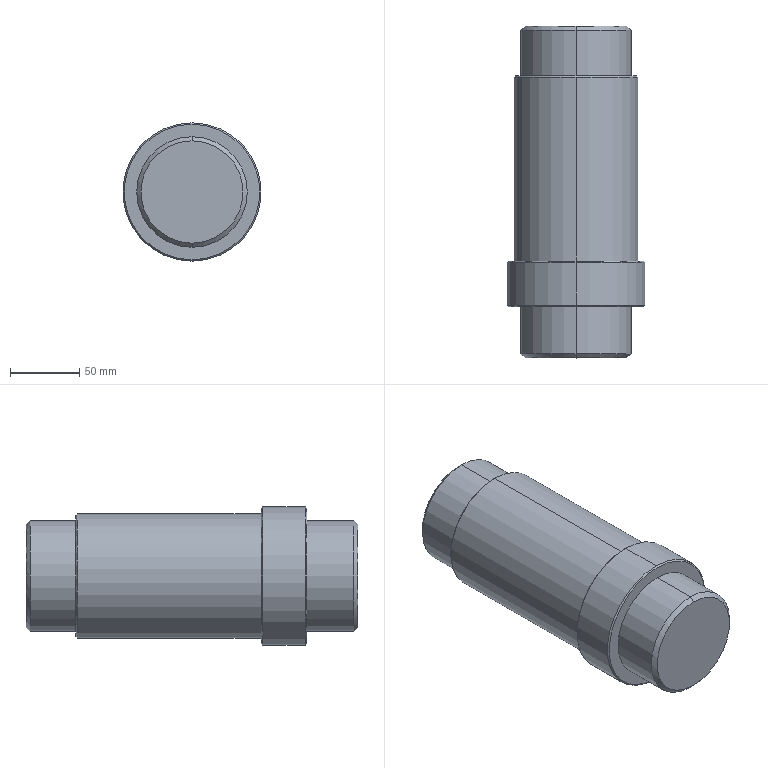Part | SolidWorks | features ICE 3, Chamfer 2, Extrusion 1 | 1 solid | 23 faces | box 100 x 240 x 100 mm | volume 1475933 mm3 | cone 10 | cylinder 8 | plane 5 | commonest cylinder face diameters 80 x4 90 x2 100 x2
STEP:
#1=CARTESIAN_POINT('',(0.,-50.,49.));
#2=VERTEX_POINT('',#1);
#3=CARTESIAN_POINT('',(0.,-50.,-49.));
#4=VERTEX_POINT('',#3);
#5=CARTESIAN_POINT('',(0.,-50.,0.));
#6=DIRECTION('',(0.,1.,0.));
#7=DIRECTION('',(0.,0.,1.));
#8=AXIS2_PLACEMENT_3D('',#5,#6,#7);
#9=CIRCLE('',#8,49.);
#10=EDGE_CURVE('',#2,#4,#9,.T.);
#11=ORIENTED_EDGE('',*,*,#10,.F.);
#12=CARTESIAN_POINT('',(0.,-51.,50.));
#13=VERTEX_POINT('',#12);
#14=CARTESIAN_POINT('',(0.,-50.,49.));
#15=DIRECTION('',(0.,-0.7071,0.7071));
#16=VECTOR('',#15,1000.);
#17=LINE('',#14,#16);
#18=EDGE_CURVE('',#2,#13,#17,.T.);
#19=ORIENTED_EDGE('',*,*,#18,.T.);
#20=CARTESIAN_POINT('',(0.,-51.,-50.));
#21=VERTEX_POINT('',#20);
#22=CARTESIAN_POINT('',(0.,-51.,0.));
#23=DIRECTION('',(0.,-1.,0.));
#24=DIRECTION('',(0.,0.,1.));
#25=AXIS2_PLACEMENT_3D('',#22,#23,#24);
#26=CIRCLE('',#25,50.);
#27=EDGE_CURVE('',#21,#13,#26,.T.);
#28=ORIENTED_EDGE('',*,*,#27,.F.);
#29=CARTESIAN_POINT('',(0.,-50.,-49.));
#30=DIRECTION('',(0.,-0.7071,-0.7071));
#31=VECTOR('',#30,1000.);
#32=LINE('',#29,#31);
#33=EDGE_CURVE('',#4,#21,#32,.T.);
#34=ORIENTED_EDGE('',*,*,#33,.F.);
#35=EDGE_LOOP('',(#11,#19,#28,#34));
#36=FACE_OUTER_BOUND('',#35,.T.);
#37=CARTESIAN_POINT('',(0.,-50.,0.));
#38=DIRECTION('',(0.,-1.,0.));
#39=DIRECTION('',(0.,0.,-1.));
#40=AXIS2_PLACEMENT_3D('',#37,#38,#39);
#41=CONICAL_SURFACE('',#40,49.,0.7854);
#42=ADVANCED_FACE('',(#36),#41,.T.);
#43=CARTESIAN_POINT('',(0.,-83.,-49.));
#44=VERTEX_POINT('',#43);
#45=CARTESIAN_POINT('',(0.,-83.,49.));
#46=VERTEX_POINT('',#45);
#47=CARTESIAN_POINT('',(0.,-83.,0.));
#48=DIRECTION('',(0.,-1.,0.));
#49=DIRECTION('',(0.,0.,-1.));
#50=AXIS2_PLACEMENT_3D('',#47,#48,#49);
#51=CIRCLE('',#50,49.);
#52=EDGE_CURVE('',#44,#46,#51,.T.);
#53=ORIENTED_EDGE('',*,*,#52,.F.);
#54=CARTESIAN_POINT('',(0.,-82.,-50.));
#55=VERTEX_POINT('',#54);
#56=CARTESIAN_POINT('',(0.,-83.,-49.));
#57=DIRECTION('',(0.,0.7071,-0.7071));
#58=VECTOR('',#57,1000.);
#59=LINE('',#56,#58);
#60=EDGE_CURVE('',#44,#55,#59,.T.);
#61=ORIENTED_EDGE('',*,*,#60,.T.);
#62=CARTESIAN_POINT('',(0.,-82.,50.));
#63=VERTEX_POINT('',#62);
#64=CARTESIAN_POINT('',(0.,-82.,0.));
#65=DIRECTION('',(0.,1.,0.));
#66=DIRECTION('',(0.,0.,-1.));
#67=AXIS2_PLACEMENT_3D('',#64,#65,#66);
#68=CIRCLE('',#67,50.);
#69=EDGE_CURVE('',#63,#55,#68,.T.);
#70=ORIENTED_EDGE('',*,*,#69,.F.);
#71=CARTESIAN_POINT('',(0.,-83.,49.));
#72=DIRECTION('',(0.,0.7071,0.7071));
#73=VECTOR('',#72,1000.);
#74=LINE('',#71,#73);
#75=EDGE_CURVE('',#46,#63,#74,.T.);
#76=ORIENTED_EDGE('',*,*,#75,.F.);
#77=EDGE_LOOP('',(#53,#61,#70,#76));
#78=FACE_OUTER_BOUND('',#77,.T.);
#79=CARTESIAN_POINT('',(0.,-83.,0.));
#80=DIRECTION('',(0.,1.,0.));
#81=DIRECTION('',(0.,0.,1.));
#82=AXIS2_PLACEMENT_3D('',#79,#80,#81);
#83=CONICAL_SURFACE('',#82,49.,0.7854);
#84=ADVANCED_FACE('',(#78),#83,.T.);
#85=CARTESIAN_POINT('',(0.,84.,44.));
#86=VERTEX_POINT('',#85);
#87=CARTESIAN_POINT('',(0.,84.,-44.));
#88=VERTEX_POINT('',#87);
#89=CARTESIAN_POINT('',(0.,84.,0.));
#90=DIRECTION('',(0.,1.,0.));
#91=DIRECTION('',(0.,0.,1.));
#92=AXIS2_PLACEMENT_3D('',#89,#90,#91);
#93=CIRCLE('',#92,44.);
#94=EDGE_CURVE('',#86,#88,#93,.T.);
#95=ORIENTED_EDGE('',*,*,#94,.F.);
#96=CARTESIAN_POINT('',(0.,83.,45.));
#97=VERTEX_POINT('',#96);
#98=CARTESIAN_POINT('',(0.,84.,44.));
#99=DIRECTION('',(0.,-0.7071,0.7071));
#100=VECTOR('',#99,1000.);
#101=LINE('',#98,#100);
#102=EDGE_CURVE('',#86,#97,#101,.T.);
#103=ORIENTED_EDGE('',*,*,#102,.T.);
#104=CARTESIAN_POINT('',(0.,83.,-45.));
#105=VERTEX_POINT('',#104);
#106=CARTESIAN_POINT('',(0.,83.,0.));
#107=DIRECTION('',(0.,-1.,0.));
#108=DIRECTION('',(0.,0.,1.));
#109=AXIS2_PLACEMENT_3D('',#106,#107,#108);
#110=CIRCLE('',#109,45.);
#111=EDGE_CURVE('',#105,#97,#110,.T.);
#112=ORIENTED_EDGE('',*,*,#111,.F.);
#113=CARTESIAN_POINT('',(0.,84.,-44.));
#114=DIRECTION('',(0.,-0.7071,-0.7071));
#115=VECTOR('',#114,1000.);
#116=LINE('',#113,#115);
#117=EDGE_CURVE('',#88,#105,#116,.T.);
#118=ORIENTED_EDGE('',*,*,#117,.F.);
#119=EDGE_LOOP('',(#95,#103,#112,#118));
#120=FACE_OUTER_BOUND('',#119,.T.);
#121=CARTESIAN_POINT('',(0.,84.,0.));
#122=DIRECTION('',(0.,-1.,0.));
#123=DIRECTION('',(0.,0.,-1.));
#124=AXIS2_PLACEMENT_3D('',#121,#122,#123);
#125=CONICAL_SURFACE('',#124,44.,0.7854);
#126=ADVANCED_FACE('',(#120),#125,.T.);
#127=CARTESIAN_POINT('',(0.,120.,37.));
#128=VERTEX_POINT('',#127);
#129=CARTESIAN_POINT('',(0.,120.,-37.));
#130=VERTEX_POINT('',#129);
#131=CARTESIAN_POINT('',(0.,120.,0.));
#132=DIRECTION('',(0.,1.,0.));
#133=DIRECTION('',(0.,0.,1.));
#134=AXIS2_PLACEMENT_3D('',#131,#132,#133);
#135=CIRCLE('',#134,37.);
#136=EDGE_CURVE('',#128,#130,#135,.T.);
#137=ORIENTED_EDGE('',*,*,#136,.F.);
#138=CARTESIAN_POINT('',(0.,117.,40.));
#139=VERTEX_POINT('',#138);
#140=CARTESIAN_POINT('',(0.,120.,37.));
#141=DIRECTION('',(0.,-0.7071,0.7071));
#142=VECTOR('',#141,1000.);
#143=LINE('',#140,#142);
#144=EDGE_CURVE('',#128,#139,#143,.T.);
#145=ORIENTED_EDGE('',*,*,#144,.T.);
#146=CARTESIAN_POINT('',(0.,117.,-40.));
#147=VERTEX_POINT('',#146);
#148=CARTESIAN_POINT('',(0.,117.,0.));
#149=DIRECTION('',(0.,-1.,0.));
#150=DIRECTION('',(0.,0.,1.));
#151=AXIS2_PLACEMENT_3D('',#148,#149,#150);
#152=CIRCLE('',#151,40.);
#153=EDGE_CURVE('',#147,#139,#152,.T.);
#154=ORIENTED_EDGE('',*,*,#153,.F.);
#155=CARTESIAN_POINT('',(0.,120.,-37.));
#156=DIRECTION('',(0.,-0.7071,-0.7071));
#157=VECTOR('',#156,1000.);
#158=LINE('',#155,#157);
#159=EDGE_CURVE('',#130,#147,#158,.T.);
#160=ORIENTED_EDGE('',*,*,#159,.F.);
#161=EDGE_LOOP('',(#137,#145,#154,#160));
#162=FACE_OUTER_BOUND('',#161,.T.);
#163=CARTESIAN_POINT('',(0.,120.,0.));
#164=DIRECTION('',(0.,-1.,0.));
#165=DIRECTION('',(0.,0.,-1.));
#166=AXIS2_PLACEMENT_3D('',#163,#164,#165);
#167=CONICAL_SURFACE('',#166,37.,0.7854);
#168=ADVANCED_FACE('',(#162),#167,.T.);
#169=CARTESIAN_POINT('',(0.,-120.,-37.));
#170=VERTEX_POINT('',#169);
#171=CARTESIAN_POINT('',(0.,-120.,37.));
#172=VERTEX_POINT('',#171);
#173=CARTESIAN_POINT('',(0.,-120.,0.));
#174=DIRECTION('',(0.,-1.,0.));
#175=DIRECTION('',(0.,0.,1.));
#176=AXIS2_PLACEMENT_3D('',#173,#174,#175);
#177=CIRCLE('',#176,37.);
#178=EDGE_CURVE('',#170,#172,#177,.T.);
#179=ORIENTED_EDGE('',*,*,#178,.F.);
#180=CARTESIAN_POINT('',(0.,-117.,-40.));
#181=VERTEX_POINT('',#180);
#182=CARTESIAN_POINT('',(0.,-120.,-37.));
#183=DIRECTION('',(0.,0.7071,-0.7071));
#184=VECTOR('',#183,1000.);
#185=LINE('',#182,#184);
#186=EDGE_CURVE('',#170,#181,#185,.T.);
#187=ORIENTED_EDGE('',*,*,#186,.T.);
#188=CARTESIAN_POINT('',(0.,-117.,40.));
#189=VERTEX_POINT('',#188);
#190=CARTESIAN_POINT('',(0.,-117.,0.));
#191=DIRECTION('',(0.,1.,0.));
#192=DIRECTION('',(0.,0.,1.));
#193=AXIS2_PLACEMENT_3D('',#190,#191,#192);
#194=CIRCLE('',#193,40.);
#195=EDGE_CURVE('',#189,#181,#194,.T.);
#196=ORIENTED_EDGE('',*,*,#195,.F.);
#197=CARTESIAN_POINT('',(0.,-120.,37.));
#198=DIRECTION('',(0.,0.7071,0.7071));
#199=VECTOR('',#198,1000.);
#200=LINE('',#197,#199);
#201=EDGE_CURVE('',#172,#189,#200,.T.);
#202=ORIENTED_EDGE('',*,*,#201,.F.);
#203=EDGE_LOOP('',(#179,#187,#196,#202));
#204=FACE_OUTER_BOUND('',#203,.T.);
#205=CARTESIAN_POINT('',(0.,-120.,0.));
#206=DIRECTION('',(0.,1.,0.));
#207=DIRECTION('',(0.,0.,1.));
#208=AXIS2_PLACEMENT_3D('',#205,#206,#207);
#209=CONICAL_SURFACE('',#208,37.,0.7854);
#210=ADVANCED_FACE('',(#204),#209,.T.);
#211=CARTESIAN_POINT('',(0.,84.,40.));
#212=VERTEX_POINT('',#211);
#213=CARTESIAN_POINT('',(0.,84.,-40.));
#214=VERTEX_POINT('',#213);
#215=CARTESIAN_POINT('',(0.,84.,0.));
#216=DIRECTION('',(0.,1.,0.));
#217=DIRECTION('',(0.,0.,1.));
#218=AXIS2_PLACEMENT_3D('',#215,#216,#217);
#219=CIRCLE('',#218,40.);
#220=EDGE_CURVE('',#212,#214,#219,.T.);
#221=ORIENTED_EDGE('',*,*,#220,.T.);
#222=CARTESIAN_POINT('',(0.,84.,-40.));
#223=DIRECTION('',(0.,1.,0.));
#224=VECTOR('',#223,1000.);
#225=LINE('',#222,#224);
#226=EDGE_CURVE('',#214,#147,#225,.T.);
#227=ORIENTED_EDGE('',*,*,#226,.T.);
#228=ORIENTED_EDGE('',*,*,#153,.T.);
#229=CARTESIAN_POINT('',(0.,84.,40.));
#230=DIRECTION('',(0.,1.,0.));
#231=VECTOR('',#230,1000.);
#232=LINE('',#229,#231);
#233=EDGE_CURVE('',#212,#139,#232,.T.);
#234=ORIENTED_EDGE('',*,*,#233,.F.);
#235=EDGE_LOOP('',(#221,#227,#228,#234));
#236=FACE_OUTER_BOUND('',#235,.T.);
#237=CARTESIAN_POINT('',(0.,84.,0.));
#238=DIRECTION('',(0.,1.,0.));
#239=DIRECTION('',(0.,0.,1.));
#240=AXIS2_PLACEMENT_3D('',#237,#238,#239);
#241=CYLINDRICAL_SURFACE('',#240,40.);
#242=ADVANCED_FACE('',(#236),#241,.T.);
#243=CARTESIAN_POINT('',(0.,-50.,45.));
#244=VERTEX_POINT('',#243);
#245=CARTESIAN_POINT('',(0.,-50.,-45.));
#246=VERTEX_POINT('',#245);
#247=CARTESIAN_POINT('',(0.,-50.,0.));
#248=DIRECTION('',(0.,1.,0.));
#249=DIRECTION('',(0.,0.,1.));
#250=AXIS2_PLACEMENT_3D('',#247,#248,#249);
#251=CIRCLE('',#250,45.);
#252=EDGE_CURVE('',#244,#246,#251,.T.);
#253=ORIENTED_EDGE('',*,*,#252,.T.);
#254=CARTESIAN_POINT('',(0.,-50.,-45.));
#255=DIRECTION('',(0.,1.,0.));
#256=VECTOR('',#255,1000.);
#257=LINE('',#254,#256);
#258=EDGE_CURVE('',#246,#105,#257,.T.);
#259=ORIENTED_EDGE('',*,*,#258,.T.);
#260=ORIENTED_EDGE('',*,*,#111,.T.);
#261=CARTESIAN_POINT('',(0.,-50.,45.));
#262=DIRECTION('',(0.,1.,0.));
#263=VECTOR('',#262,1000.);
#264=LINE('',#261,#263);
#265=EDGE_CURVE('',#244,#97,#264,.T.);
#266=ORIENTED_EDGE('',*,*,#265,.F.);
#267=EDGE_LOOP('',(#253,#259,#260,#266));
#268=FACE_OUTER_BOUND('',#267,.T.);
#269=CARTESIAN_POINT('',(0.,-50.,0.));
#270=DIRECTION('',(0.,1.,0.));
#271=DIRECTION('',(0.,0.,1.));
#272=AXIS2_PLACEMENT_3D('',#269,#270,#271);
#273=CYLINDRICAL_SURFACE('',#272,45.);
#274=ADVANCED_FACE('',(#268),#273,.T.);
#275=CARTESIAN_POINT('',(0.,-83.,-40.));
#276=VERTEX_POINT('',#275);
#277=CARTESIAN_POINT('',(0.,-83.,40.));
#278=VERTEX_POINT('',#277);
#279=CARTESIAN_POINT('',(0.,-83.,0.));
#280=DIRECTION('',(0.,-1.,0.));
#281=DIRECTION('',(0.,0.,-1.));
#282=AXIS2_PLACEMENT_3D('',#279,#280,#281);
#283=CIRCLE('',#282,40.);
#284=EDGE_CURVE('',#276,#278,#283,.T.);
#285=ORIENTED_EDGE('',*,*,#284,.T.);
#286=CARTESIAN_POINT('',(0.,-83.,40.));
#287=DIRECTION('',(0.,-1.,0.));
#288=VECTOR('',#287,1000.);
#289=LINE('',#286,#288);
#290=EDGE_CURVE('',#278,#189,#289,.T.);
#291=ORIENTED_EDGE('',*,*,#290,.T.);
#292=ORIENTED_EDGE('',*,*,#195,.T.);
#293=CARTESIAN_POINT('',(0.,-83.,-40.));
#294=DIRECTION('',(0.,-1.,0.));
#295=VECTOR('',#294,1000.);
#296=LINE('',#293,#295);
#297=EDGE_CURVE('',#276,#181,#296,.T.);
#298=ORIENTED_EDGE('',*,*,#297,.F.);
#299=EDGE_LOOP('',(#285,#291,#292,#298));
#300=FACE_OUTER_BOUND('',#299,.T.);
#301=CARTESIAN_POINT('',(0.,-83.,0.));
#302=DIRECTION('',(0.,-1.,0.));
#303=DIRECTION('',(0.,0.,-1.));
#304=AXIS2_PLACEMENT_3D('',#301,#302,#303);
#305=CYLINDRICAL_SURFACE('',#304,40.);
#306=ADVANCED_FACE('',(#300),#305,.T.);
#307=ORIENTED_EDGE('',*,*,#27,.T.);
#308=CARTESIAN_POINT('',(0.,120.,50.));
#309=DIRECTION('',(0.,-1.,0.));
#310=VECTOR('',#309,1000.);
#311=LINE('',#308,#310);
#312=EDGE_CURVE('',#13,#63,#311,.T.);
#313=ORIENTED_EDGE('',*,*,#312,.T.);
#314=ORIENTED_EDGE('',*,*,#69,.T.);
#315=CARTESIAN_POINT('',(0.,120.,-50.));
#316=DIRECTION('',(0.,-1.,0.));
#317=VECTOR('',#316,1000.);
#318=LINE('',#315,#317);
#319=EDGE_CURVE('',#21,#55,#318,.T.);
#320=ORIENTED_EDGE('',*,*,#319,.F.);
#321=EDGE_LOOP('',(#307,#313,#314,#320));
#322=FACE_OUTER_BOUND('',#321,.T.);
#323=CARTESIAN_POINT('',(0.,120.,0.));
#324=DIRECTION('',(0.,-1.,0.));
#325=DIRECTION('',(0.,0.,-1.));
#326=AXIS2_PLACEMENT_3D('',#323,#324,#325);
#327=CYLINDRICAL_SURFACE('',#326,50.);
#328=ADVANCED_FACE('',(#322),#327,.T.);
#329=ORIENTED_EDGE('',*,*,#312,.F.);
#330=CARTESIAN_POINT('',(0.,-51.,0.));
#331=DIRECTION('',(0.,-1.,0.));
#332=DIRECTION('',(0.,0.,1.));
#333=AXIS2_PLACEMENT_3D('',#330,#331,#332);
#334=CIRCLE('',#333,50.);
#335=EDGE_CURVE('',#13,#21,#334,.T.);
#336=ORIENTED_EDGE('',*,*,#335,.T.);
#337=ORIENTED_EDGE('',*,*,#319,.T.);
#338=CARTESIAN_POINT('',(0.,-82.,0.));
#339=DIRECTION('',(0.,1.,0.));
#340=DIRECTION('',(0.,0.,-1.));
#341=AXIS2_PLACEMENT_3D('',#338,#339,#340);
#342=CIRCLE('',#341,50.);
#343=EDGE_CURVE('',#55,#63,#342,.T.);
#344=ORIENTED_EDGE('',*,*,#343,.T.);
#345=EDGE_LOOP('',(#329,#336,#337,#344));
#346=FACE_OUTER_BOUND('',#345,.T.);
#347=CARTESIAN_POINT('',(0.,120.,0.));
#348=DIRECTION('',(0.,-1.,0.));
#349=DIRECTION('',(0.,0.,-1.));
#350=AXIS2_PLACEMENT_3D('',#347,#348,#349);
#351=CYLINDRICAL_SURFACE('',#350,50.);
#352=ADVANCED_FACE('',(#346),#351,.T.);
#353=CARTESIAN_POINT('',(0.,-83.,0.));
#354=DIRECTION('',(0.,-1.,0.));
#355=DIRECTION('',(0.,0.,-1.));
#356=AXIS2_PLACEMENT_3D('',#353,#354,#355);
#357=CIRCLE('',#356,49.);
#358=EDGE_CURVE('',#46,#44,#357,.T.);
#359=ORIENTED_EDGE('',*,*,#358,.T.);
#360=ORIENTED_EDGE('',*,*,#52,.T.);
#361=EDGE_LOOP('',(#359,#360));
#362=FACE_OUTER_BOUND('',#361,.T.);
#363=ORIENTED_EDGE('',*,*,#284,.F.);
#364=CARTESIAN_POINT('',(0.,-83.,0.));
#365=DIRECTION('',(0.,-1.,0.));
#366=DIRECTION('',(0.,0.,-1.));
#367=AXIS2_PLACEMENT_3D('',#364,#365,#366);
#368=CIRCLE('',#367,40.);
#369=EDGE_CURVE('',#278,#276,#368,.T.);
#370=ORIENTED_EDGE('',*,*,#369,.F.);
#371=EDGE_LOOP('',(#363,#370));
#372=FACE_BOUND('',#371,.T.);
#373=CARTESIAN_POINT('',(0.,-83.,0.));
#374=DIRECTION('',(0.,-1.,0.));
#375=DIRECTION('',(0.,0.,-1.));
#376=AXIS2_PLACEMENT_3D('',#373,#374,#375);
#377=PLANE('',#376);
#378=ADVANCED_FACE('',(#362,#372),#377,.T.);
#379=ORIENTED_EDGE('',*,*,#290,.F.);
#380=ORIENTED_EDGE('',*,*,#369,.T.);
#381=ORIENTED_EDGE('',*,*,#297,.T.);
#382=CARTESIAN_POINT('',(0.,-117.,0.));
#383=DIRECTION('',(0.,1.,0.));
#384=DIRECTION('',(0.,0.,1.));
#385=AXIS2_PLACEMENT_3D('',#382,#383,#384);
#386=CIRCLE('',#385,40.);
#387=EDGE_CURVE('',#181,#189,#386,.T.);
#388=ORIENTED_EDGE('',*,*,#387,.T.);
#389=EDGE_LOOP('',(#379,#380,#381,#388));
#390=FACE_OUTER_BOUND('',#389,.T.);
#391=CARTESIAN_POINT('',(0.,-83.,0.));
#392=DIRECTION('',(0.,-1.,0.));
#393=DIRECTION('',(0.,0.,-1.));
#394=AXIS2_PLACEMENT_3D('',#391,#392,#393);
#395=CYLINDRICAL_SURFACE('',#394,40.);
#396=ADVANCED_FACE('',(#390),#395,.T.);
#397=CARTESIAN_POINT('',(0.,-120.,0.));
#398=DIRECTION('',(0.,-1.,0.));
#399=DIRECTION('',(0.,0.,1.));
#400=AXIS2_PLACEMENT_3D('',#397,#398,#399);
#401=CIRCLE('',#400,37.);
#402=EDGE_CURVE('',#172,#170,#401,.T.);
#403=ORIENTED_EDGE('',*,*,#402,.T.);
#404=ORIENTED_EDGE('',*,*,#178,.T.);
#405=EDGE_LOOP('',(#403,#404));
#406=FACE_OUTER_BOUND('',#405,.T.);
#407=CARTESIAN_POINT('',(0.,-120.,0.));
#408=DIRECTION('',(0.,1.,0.));
#409=DIRECTION('',(0.,0.,1.));
#410=AXIS2_PLACEMENT_3D('',#407,#408,#409);
#411=PLANE('',#410);
#412=ADVANCED_FACE('',(#406),#411,.F.);
#413=CARTESIAN_POINT('',(0.,-50.,0.));
#414=DIRECTION('',(0.,1.,0.));
#415=DIRECTION('',(0.,0.,1.));
#416=AXIS2_PLACEMENT_3D('',#413,#414,#415);
#417=CIRCLE('',#416,49.);
#418=EDGE_CURVE('',#4,#2,#417,.T.);
#419=ORIENTED_EDGE('',*,*,#418,.T.);
#420=ORIENTED_EDGE('',*,*,#10,.T.);
#421=EDGE_LOOP('',(#419,#420));
#422=FACE_OUTER_BOUND('',#421,.T.);
#423=ORIENTED_EDGE('',*,*,#252,.F.);
#424=CARTESIAN_POINT('',(0.,-50.,0.));
#425=DIRECTION('',(0.,1.,0.));
#426=DIRECTION('',(0.,0.,1.));
#427=AXIS2_PLACEMENT_3D('',#424,#425,#426);
#428=CIRCLE('',#427,45.);
#429=EDGE_CURVE('',#246,#244,#428,.T.);
#430=ORIENTED_EDGE('',*,*,#429,.F.);
#431=EDGE_LOOP('',(#423,#430));
#432=FACE_BOUND('',#431,.T.);
#433=CARTESIAN_POINT('',(0.,-50.,0.));
#434=DIRECTION('',(0.,1.,0.));
#435=DIRECTION('',(0.,0.,1.));
#436=AXIS2_PLACEMENT_3D('',#433,#434,#435);
#437=PLANE('',#436);
#438=ADVANCED_FACE('',(#422,#432),#437,.T.);
#439=ORIENTED_EDGE('',*,*,#258,.F.);
#440=ORIENTED_EDGE('',*,*,#429,.T.);
#441=ORIENTED_EDGE('',*,*,#265,.T.);
#442=CARTESIAN_POINT('',(0.,83.,0.));
#443=DIRECTION('',(0.,-1.,0.));
#444=DIRECTION('',(0.,0.,1.));
#445=AXIS2_PLACEMENT_3D('',#442,#443,#444);
#446=CIRCLE('',#445,45.);
#447=EDGE_CURVE('',#97,#105,#446,.T.);
#448=ORIENTED_EDGE('',*,*,#447,.T.);
#449=EDGE_LOOP('',(#439,#440,#441,#448));
#450=FACE_OUTER_BOUND('',#449,.T.);
#451=CARTESIAN_POINT('',(0.,-50.,0.));
#452=DIRECTION('',(0.,1.,0.));
#453=DIRECTION('',(0.,0.,1.));
#454=AXIS2_PLACEMENT_3D('',#451,#452,#453);
#455=CYLINDRICAL_SURFACE('',#454,45.);
#456=ADVANCED_FACE('',(#450),#455,.T.);
#457=CARTESIAN_POINT('',(0.,120.,0.));
#458=DIRECTION('',(0.,1.,0.));
#459=DIRECTION('',(0.,0.,1.));
#460=AXIS2_PLACEMENT_3D('',#457,#458,#459);
#461=CIRCLE('',#460,37.);
#462=EDGE_CURVE('',#130,#128,#461,.T.);
#463=ORIENTED_EDGE('',*,*,#462,.T.);
#464=ORIENTED_EDGE('',*,*,#136,.T.);
#465=EDGE_LOOP('',(#463,#464));
#466=FACE_OUTER_BOUND('',#465,.T.);
#467=CARTESIAN_POINT('',(0.,120.,0.));
#468=DIRECTION('',(0.,1.,0.));
#469=DIRECTION('',(0.,0.,1.));
#470=AXIS2_PLACEMENT_3D('',#467,#468,#469);
#471=PLANE('',#470);
#472=ADVANCED_FACE('',(#466),#471,.T.);
#473=ORIENTED_EDGE('',*,*,#226,.F.);
#474=CARTESIAN_POINT('',(0.,84.,0.));
#475=DIRECTION('',(0.,1.,0.));
#476=DIRECTION('',(0.,0.,1.));
#477=AXIS2_PLACEMENT_3D('',#474,#475,#476);
#478=CIRCLE('',#477,40.);
#479=EDGE_CURVE('',#214,#212,#478,.T.);
#480=ORIENTED_EDGE('',*,*,#479,.T.);
#481=ORIENTED_EDGE('',*,*,#233,.T.);
#482=CARTESIAN_POINT('',(0.,117.,0.));
#483=DIRECTION('',(0.,-1.,0.));
#484=DIRECTION('',(0.,0.,1.));
#485=AXIS2_PLACEMENT_3D('',#482,#483,#484);
#486=CIRCLE('',#485,40.);
#487=EDGE_CURVE('',#139,#147,#486,.T.);
#488=ORIENTED_EDGE('',*,*,#487,.T.);
#489=EDGE_LOOP('',(#473,#480,#481,#488));
#490=FACE_OUTER_BOUND('',#489,.T.);
#491=CARTESIAN_POINT('',(0.,84.,0.));
#492=DIRECTION('',(0.,1.,0.));
#493=DIRECTION('',(0.,0.,1.));
#494=AXIS2_PLACEMENT_3D('',#491,#492,#493);
#495=CYLINDRICAL_SURFACE('',#494,40.);
#496=ADVANCED_FACE('',(#490),#495,.T.);
#497=CARTESIAN_POINT('',(0.,84.,0.));
#498=DIRECTION('',(0.,1.,0.));
#499=DIRECTION('',(0.,0.,1.));
#500=AXIS2_PLACEMENT_3D('',#497,#498,#499);
#501=CIRCLE('',#500,44.);
#502=EDGE_CURVE('',#88,#86,#501,.T.);
#503=ORIENTED_EDGE('',*,*,#502,.T.);
#504=ORIENTED_EDGE('',*,*,#94,.T.);
#505=EDGE_LOOP('',(#503,#504));
#506=FACE_OUTER_BOUND('',#505,.T.);
#507=ORIENTED_EDGE('',*,*,#220,.F.);
#508=ORIENTED_EDGE('',*,*,#479,.F.);
#509=EDGE_LOOP('',(#507,#508));
#510=FACE_BOUND('',#509,.T.);
#511=CARTESIAN_POINT('',(0.,84.,0.));
#512=DIRECTION('',(0.,1.,0.));
#513=DIRECTION('',(0.,0.,1.));
#514=AXIS2_PLACEMENT_3D('',#511,#512,#513);
#515=PLANE('',#514);
#516=ADVANCED_FACE('',(#506,#510),#515,.T.);
#517=ORIENTED_EDGE('',*,*,#186,.F.);
#518=ORIENTED_EDGE('',*,*,#402,.F.);
#519=ORIENTED_EDGE('',*,*,#201,.T.);
#520=ORIENTED_EDGE('',*,*,#387,.F.);
#521=EDGE_LOOP('',(#517,#518,#519,#520));
#522=FACE_OUTER_BOUND('',#521,.T.);
#523=CARTESIAN_POINT('',(0.,-120.,0.));
#524=DIRECTION('',(0.,1.,0.));
#525=DIRECTION('',(0.,0.,1.));
#526=AXIS2_PLACEMENT_3D('',#523,#524,#525);
#527=CONICAL_SURFACE('',#526,37.,0.7854);
#528=ADVANCED_FACE('',(#522),#527,.T.);
#529=ORIENTED_EDGE('',*,*,#144,.F.);
#530=ORIENTED_EDGE('',*,*,#462,.F.);
#531=ORIENTED_EDGE('',*,*,#159,.T.);
#532=ORIENTED_EDGE('',*,*,#487,.F.);
#533=EDGE_LOOP('',(#529,#530,#531,#532));
#534=FACE_OUTER_BOUND('',#533,.T.);
#535=CARTESIAN_POINT('',(0.,120.,0.));
#536=DIRECTION('',(0.,-1.,0.));
#537=DIRECTION('',(0.,0.,-1.));
#538=AXIS2_PLACEMENT_3D('',#535,#536,#537);
#539=CONICAL_SURFACE('',#538,37.,0.7854);
#540=ADVANCED_FACE('',(#534),#539,.T.);
#541=ORIENTED_EDGE('',*,*,#102,.F.);
#542=ORIENTED_EDGE('',*,*,#502,.F.);
#543=ORIENTED_EDGE('',*,*,#117,.T.);
#544=ORIENTED_EDGE('',*,*,#447,.F.);
#545=EDGE_LOOP('',(#541,#542,#543,#544));
#546=FACE_OUTER_BOUND('',#545,.T.);
#547=CARTESIAN_POINT('',(0.,84.,0.));
#548=DIRECTION('',(0.,-1.,0.));
#549=DIRECTION('',(0.,0.,-1.));
#550=AXIS2_PLACEMENT_3D('',#547,#548,#549);
#551=CONICAL_SURFACE('',#550,44.,0.7854);
#552=ADVANCED_FACE('',(#546),#551,.T.);
#553=ORIENTED_EDGE('',*,*,#60,.F.);
#554=ORIENTED_EDGE('',*,*,#358,.F.);
#555=ORIENTED_EDGE('',*,*,#75,.T.);
#556=ORIENTED_EDGE('',*,*,#343,.F.);
#557=EDGE_LOOP('',(#553,#554,#555,#556));
#558=FACE_OUTER_BOUND('',#557,.T.);
#559=CARTESIAN_POINT('',(0.,-83.,0.));
#560=DIRECTION('',(0.,1.,0.));
#561=DIRECTION('',(0.,0.,1.));
#562=AXIS2_PLACEMENT_3D('',#559,#560,#561);
#563=CONICAL_SURFACE('',#562,49.,0.7854);
#564=ADVANCED_FACE('',(#558),#563,.T.);
#565=ORIENTED_EDGE('',*,*,#18,.F.);
#566=ORIENTED_EDGE('',*,*,#418,.F.);
#567=ORIENTED_EDGE('',*,*,#33,.T.);
#568=ORIENTED_EDGE('',*,*,#335,.F.);
#569=EDGE_LOOP('',(#565,#566,#567,#568));
#570=FACE_OUTER_BOUND('',#569,.T.);
#571=CARTESIAN_POINT('',(0.,-50.,0.));
#572=DIRECTION('',(0.,-1.,0.));
#573=DIRECTION('',(0.,0.,-1.));
#574=AXIS2_PLACEMENT_3D('',#571,#572,#573);
#575=CONICAL_SURFACE('',#574,49.,0.7854);
#576=ADVANCED_FACE('',(#570),#575,.T.);
#577=CLOSED_SHELL('',(#42,#84,#126,#168,#210,#242,#274,#306,#328,#352,#378,#396,#412,#438,#456,#472,#496,#516,#528,#540,#552,#564,#576));
#578=MANIFOLD_SOLID_BREP('',#577);
#579=CARTESIAN_POINT('',(0.,0.,0.));
#580=DIRECTION('',(0.,0.,1.));
#581=DIRECTION('',(1.,0.,0.));
#582=AXIS2_PLACEMENT_3D('',#579,#580,#581);
#583=(LENGTH_UNIT()NAMED_UNIT(*)SI_UNIT(.MILLI.,.METRE.));
#584=UNCERTAINTY_MEASURE_WITH_UNIT(LENGTH_MEASURE(0.00001),#583,'','');
#585=(NAMED_UNIT(*)PLANE_ANGLE_UNIT()SI_UNIT($,.RADIAN.));
#586=(NAMED_UNIT(*)SI_UNIT($,.STERADIAN.)SOLID_ANGLE_UNIT());
#587=(GEOMETRIC_REPRESENTATION_CONTEXT(3)GLOBAL_UNCERTAINTY_ASSIGNED_CONTEXT((#584))GLOBAL_UNIT_ASSIGNED_CONTEXT((#583,#585,#586))REPRESENTATION_CONTEXT('',''));
#588=ADVANCED_BREP_SHAPE_REPRESENTATION('',(#578,#582),#587);